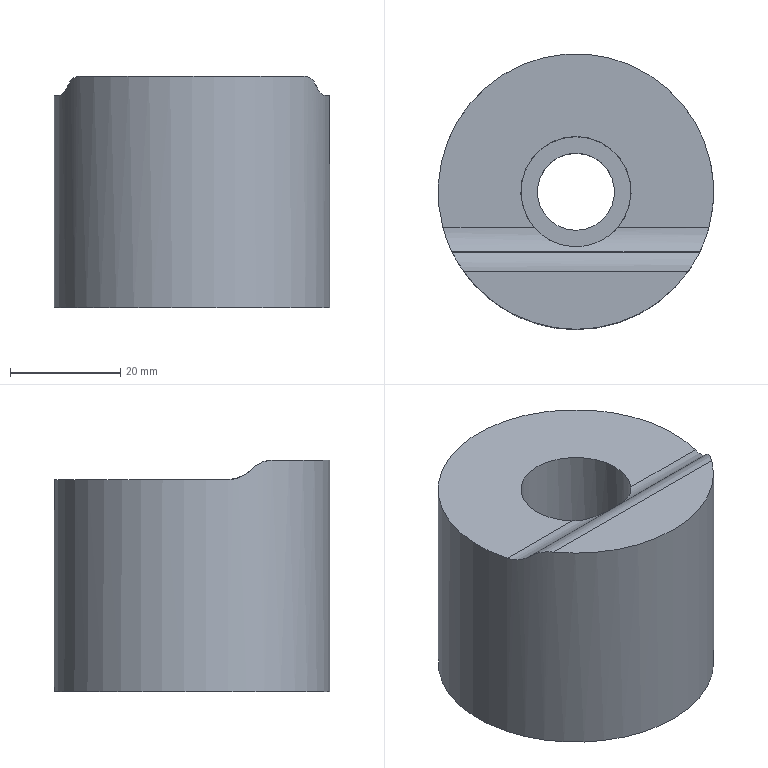Part | NX | features solid 2 | 1 solid | 10 faces | box 50 x 50 x 42.008 mm | volume 68335 mm3 | cylinder 5 | plane 5 | commonest cylinder face diameters 10 x1 12 x1 14 x1 20 x1 50 x1
STEP:
#1=CARTESIAN_POINT('',(-225.,485.,50.));
#2=VERTEX_POINT('',#1);
#3=CARTESIAN_POINT('',(-225.,510.,50.));
#4=DIRECTION('',(0.,0.,1.));
#5=DIRECTION('',(0.,-1.,0.));
#6=AXIS2_PLACEMENT_3D('',#3,#4,#5);
#7=CIRCLE('',#6,25.);
#8=EDGE_CURVE('',#2,#2,#7,.T.);
#9=ORIENTED_EDGE('',*,*,#8,.T.);
#10=EDGE_LOOP('',(#9));
#11=FACE_BOUND('',#10,.T.);
#12=CARTESIAN_POINT('',(-245.311,495.423,92.008));
#13=VERTEX_POINT('',#12);
#14=CARTESIAN_POINT('',(-204.689,495.423,92.008));
#15=VERTEX_POINT('',#14);
#16=CARTESIAN_POINT('',(-225.,510.,92.008));
#17=DIRECTION('',(0.,0.,1.));
#18=DIRECTION('',(0.,-1.,0.));
#19=AXIS2_PLACEMENT_3D('',#16,#17,#18);
#20=CIRCLE('',#19,25.);
#21=EDGE_CURVE('',#13,#15,#20,.T.);
#22=ORIENTED_EDGE('',*,*,#21,.F.);
#23=CARTESIAN_POINT('',(-247.454,499.009,90.492));
#24=VERTEX_POINT('',#23);
#25=CARTESIAN_POINT('',(-247.454,499.009,90.492));
#26=CARTESIAN_POINT('',(-246.96,497.999,91.532));
#27=CARTESIAN_POINT('',(-246.201,496.664,92.008));
#28=CARTESIAN_POINT('',(-245.311,495.423,92.008));
#29=B_SPLINE_CURVE_WITH_KNOTS('',3,(#25,#26,#27,#28),.UNSPECIFIED.,.F.,.F.,(4,4),(0.,0.004522),.UNSPECIFIED.);
#30=EDGE_CURVE('',#24,#13,#29,.T.);
#31=ORIENTED_EDGE('',*,*,#30,.F.);
#32=CARTESIAN_POINT('',(-247.533,499.171,90.326));
#33=VERTEX_POINT('',#32);
#34=CARTESIAN_POINT('',(-225.,510.,79.184));
#35=DIRECTION('',(0.,-0.7171,-0.697));
#36=DIRECTION('',(0.,0.697,-0.7171));
#37=AXIS2_PLACEMENT_3D('',#34,#35,#36);
#38=ELLIPSE('',#37,35.87,25.);
#39=EDGE_CURVE('',#24,#33,#38,.T.);
#40=ORIENTED_EDGE('',*,*,#39,.T.);
#41=CARTESIAN_POINT('',(-249.133,503.474,88.508));
#42=VERTEX_POINT('',#41);
#43=CARTESIAN_POINT('',(-247.533,499.171,90.326));
#44=CARTESIAN_POINT('',(-248.073,500.295,89.169));
#45=CARTESIAN_POINT('',(-248.689,501.831,88.508));
#46=CARTESIAN_POINT('',(-249.133,503.474,88.508));
#47=B_SPLINE_CURVE_WITH_KNOTS('',3,(#43,#44,#45,#46),.UNSPECIFIED.,.F.,.F.,(4,4),(0.,0.005031),.UNSPECIFIED.);
#48=EDGE_CURVE('',#33,#42,#47,.T.);
#49=ORIENTED_EDGE('',*,*,#48,.T.);
#50=CARTESIAN_POINT('',(-200.867,503.474,88.508));
#51=VERTEX_POINT('',#50);
#52=CARTESIAN_POINT('',(-225.,510.,88.508));
#53=DIRECTION('',(0.,0.,1.));
#54=DIRECTION('',(0.,-1.,0.));
#55=AXIS2_PLACEMENT_3D('',#52,#53,#54);
#56=CIRCLE('',#55,25.);
#57=EDGE_CURVE('',#51,#42,#56,.T.);
#58=ORIENTED_EDGE('',*,*,#57,.F.);
#59=CARTESIAN_POINT('',(-202.467,499.171,90.326));
#60=VERTEX_POINT('',#59);
#61=CARTESIAN_POINT('',(-200.867,503.474,88.508));
#62=CARTESIAN_POINT('',(-201.311,501.831,88.508));
#63=CARTESIAN_POINT('',(-201.927,500.294,89.17));
#64=CARTESIAN_POINT('',(-202.467,499.171,90.326));
#65=B_SPLINE_CURVE_WITH_KNOTS('',3,(#61,#62,#63,#64),.UNSPECIFIED.,.F.,.F.,(4,4),(0.,0.005028),.UNSPECIFIED.);
#66=EDGE_CURVE('',#51,#60,#65,.T.);
#67=ORIENTED_EDGE('',*,*,#66,.T.);
#68=CARTESIAN_POINT('',(-202.546,499.009,90.492));
#69=VERTEX_POINT('',#68);
#70=CARTESIAN_POINT('',(-225.,510.,79.184));
#71=DIRECTION('',(0.,-0.7171,-0.697));
#72=DIRECTION('',(0.,0.697,-0.7171));
#73=AXIS2_PLACEMENT_3D('',#70,#71,#72);
#74=ELLIPSE('',#73,35.87,25.);
#75=EDGE_CURVE('',#60,#69,#74,.T.);
#76=ORIENTED_EDGE('',*,*,#75,.T.);
#77=CARTESIAN_POINT('',(-204.689,495.423,92.008));
#78=CARTESIAN_POINT('',(-203.796,496.669,92.008));
#79=CARTESIAN_POINT('',(-203.043,497.993,91.538));
#80=CARTESIAN_POINT('',(-202.546,499.009,90.492));
#81=B_SPLINE_CURVE_WITH_KNOTS('',3,(#77,#78,#79,#80),.UNSPECIFIED.,.F.,.F.,(4,4),(0.,0.004516),.UNSPECIFIED.);
#82=EDGE_CURVE('',#15,#69,#81,.T.);
#83=ORIENTED_EDGE('',*,*,#82,.F.);
#84=EDGE_LOOP('',(#22,#31,#40,#49,#58,#67,#76,#83));
#85=FACE_BOUND('',#84,.T.);
#86=CARTESIAN_POINT('',(-225.,510.,100.));
#87=DIRECTION('',(0.,0.,-1.));
#88=DIRECTION('',(0.,1.,0.));
#89=AXIS2_PLACEMENT_3D('',#86,#87,#88);
#90=CYLINDRICAL_SURFACE('',#89,25.);
#91=ADVANCED_FACE('',(#11,#85),#90,.T.);
#92=CARTESIAN_POINT('',(-225.,503.,50.));
#93=VERTEX_POINT('',#92);
#94=CARTESIAN_POINT('',(-225.,510.,50.));
#95=DIRECTION('',(0.,0.,1.));
#96=DIRECTION('',(0.,-1.,0.));
#97=AXIS2_PLACEMENT_3D('',#94,#95,#96);
#98=CIRCLE('',#97,7.);
#99=EDGE_CURVE('',#93,#93,#98,.T.);
#100=ORIENTED_EDGE('',*,*,#99,.T.);
#101=EDGE_LOOP('',(#100));
#102=FACE_BOUND('',#101,.T.);
#103=ORIENTED_EDGE('',*,*,#8,.F.);
#104=EDGE_LOOP('',(#103));
#105=FACE_BOUND('',#104,.T.);
#106=CARTESIAN_POINT('',(-225.,510.,50.));
#107=DIRECTION('',(0.,0.,1.));
#108=DIRECTION('',(0.,-1.,0.));
#109=AXIS2_PLACEMENT_3D('',#106,#107,#108);
#110=PLANE('',#109);
#111=ADVANCED_FACE('',(#102,#105),#110,.F.);
#112=CARTESIAN_POINT('',(-204.689,495.423,92.008));
#113=CARTESIAN_POINT('',(-218.23,495.423,92.008));
#114=CARTESIAN_POINT('',(-231.77,495.423,92.008));
#115=CARTESIAN_POINT('',(-245.311,495.423,92.008));
#116=B_SPLINE_CURVE_WITH_KNOTS('',3,(#112,#113,#114,#115),.UNSPECIFIED.,.F.,.F.,(4,4),(0.7307,0.8175),.UNSPECIFIED.);
#117=EDGE_CURVE('',#15,#13,#116,.T.);
#118=ORIENTED_EDGE('',*,*,#117,.T.);
#119=ORIENTED_EDGE('',*,*,#21,.T.);
#120=EDGE_LOOP('',(#118,#119));
#121=FACE_BOUND('',#120,.T.);
#122=CARTESIAN_POINT('',(575.068,183.357,92.008));
#123=DIRECTION('',(0.,0.,1.));
#124=DIRECTION('',(0.,-1.,0.));
#125=AXIS2_PLACEMENT_3D('',#122,#123,#124);
#126=PLANE('',#125);
#127=ADVANCED_FACE('',(#121),#126,.T.);
#128=ORIENTED_EDGE('',*,*,#75,.F.);
#129=CARTESIAN_POINT('',(-247.533,499.171,90.326));
#130=CARTESIAN_POINT('',(-232.511,499.171,90.326));
#131=CARTESIAN_POINT('',(-217.489,499.171,90.326));
#132=CARTESIAN_POINT('',(-202.467,499.171,90.326));
#133=B_SPLINE_CURVE_WITH_KNOTS('',3,(#129,#130,#131,#132),.UNSPECIFIED.,.F.,.F.,(4,4),(0.1782,0.2748),.UNSPECIFIED.);
#134=EDGE_CURVE('',#33,#60,#133,.T.);
#135=ORIENTED_EDGE('',*,*,#134,.F.);
#136=ORIENTED_EDGE('',*,*,#39,.F.);
#137=CARTESIAN_POINT('',(-202.546,499.009,90.492));
#138=CARTESIAN_POINT('',(-217.515,499.009,90.492));
#139=CARTESIAN_POINT('',(-232.485,499.009,90.492));
#140=CARTESIAN_POINT('',(-247.454,499.009,90.492));
#141=B_SPLINE_CURVE_WITH_KNOTS('',3,(#137,#138,#139,#140),.UNSPECIFIED.,.F.,.F.,(4,4),(0.7254,0.8216),.UNSPECIFIED.);
#142=EDGE_CURVE('',#69,#24,#141,.T.);
#143=ORIENTED_EDGE('',*,*,#142,.F.);
#144=EDGE_LOOP('',(#128,#135,#136,#143));
#145=FACE_BOUND('',#144,.T.);
#146=CARTESIAN_POINT('',(-141.622,759.809,-177.845));
#147=DIRECTION('',(0.,-0.7171,-0.697));
#148=DIRECTION('',(0.,0.697,-0.7171));
#149=AXIS2_PLACEMENT_3D('',#146,#147,#148);
#150=PLANE('',#149);
#151=ADVANCED_FACE('',(#145),#150,.F.);
#152=ORIENTED_EDGE('',*,*,#117,.F.);
#153=ORIENTED_EDGE('',*,*,#82,.T.);
#154=ORIENTED_EDGE('',*,*,#142,.T.);
#155=ORIENTED_EDGE('',*,*,#30,.T.);
#156=EDGE_LOOP('',(#152,#153,#154,#155));
#157=FACE_BOUND('',#156,.T.);
#158=CARTESIAN_POINT('',(-6000330.729,495.423,87.008));
#159=DIRECTION('',(1.,0.,0.));
#160=DIRECTION('',(0.,0.,1.));
#161=AXIS2_PLACEMENT_3D('',#158,#159,#160);
#162=CYLINDRICAL_SURFACE('',#161,5.);
#163=ADVANCED_FACE('',(#157),#162,.T.);
#164=ORIENTED_EDGE('',*,*,#48,.F.);
#165=ORIENTED_EDGE('',*,*,#134,.T.);
#166=ORIENTED_EDGE('',*,*,#66,.F.);
#167=CARTESIAN_POINT('',(-217.423,503.474,88.508));
#168=VERTEX_POINT('',#167);
#169=CARTESIAN_POINT('',(-217.423,503.474,88.508));
#170=CARTESIAN_POINT('',(-211.905,503.474,88.508));
#171=CARTESIAN_POINT('',(-206.386,503.474,88.508));
#172=CARTESIAN_POINT('',(-200.867,503.474,88.508));
#173=B_SPLINE_CURVE_WITH_KNOTS('',3,(#169,#170,#171,#172),.UNSPECIFIED.,.F.,.F.,(4,4),(0.2427,0.2782),.UNSPECIFIED.);
#174=EDGE_CURVE('',#51,#168,#173,.F.);
#175=ORIENTED_EDGE('',*,*,#174,.T.);
#176=CARTESIAN_POINT('',(-232.577,503.474,88.508));
#177=VERTEX_POINT('',#176);
#178=CARTESIAN_POINT('',(-232.577,503.474,88.508));
#179=CARTESIAN_POINT('',(-231.621,502.365,88.508));
#180=CARTESIAN_POINT('',(-229.312,500.641,89.103));
#181=CARTESIAN_POINT('',(-225.005,499.681,89.871));
#182=CARTESIAN_POINT('',(-220.692,500.637,89.104));
#183=CARTESIAN_POINT('',(-218.378,502.366,88.508));
#184=CARTESIAN_POINT('',(-217.423,503.474,88.508));
#185=B_SPLINE_CURVE_WITH_KNOTS('',3,(#178,#179,#180,#181,#182,#183,#184),.UNSPECIFIED.,.F.,.F.,(4,1,1,1,4),(0.,0.004314,0.008627,0.01294,0.01725),.UNSPECIFIED.);
#186=EDGE_CURVE('',#177,#168,#185,.T.);
#187=ORIENTED_EDGE('',*,*,#186,.F.);
#188=CARTESIAN_POINT('',(-249.133,503.474,88.508));
#189=CARTESIAN_POINT('',(-243.614,503.474,88.508));
#190=CARTESIAN_POINT('',(-238.095,503.474,88.508));
#191=CARTESIAN_POINT('',(-232.577,503.474,88.508));
#192=B_SPLINE_CURVE_WITH_KNOTS('',3,(#188,#189,#190,#191),.UNSPECIFIED.,.F.,.F.,(4,4),(0.1747,0.2102),.UNSPECIFIED.);
#193=EDGE_CURVE('',#177,#42,#192,.F.);
#194=ORIENTED_EDGE('',*,*,#193,.T.);
#195=EDGE_LOOP('',(#164,#165,#166,#175,#187,#194));
#196=FACE_BOUND('',#195,.T.);
#197=CARTESIAN_POINT('',(6000135.646,503.474,94.508));
#198=DIRECTION('',(-1.,0.,0.));
#199=DIRECTION('',(0.,0.,-1.));
#200=AXIS2_PLACEMENT_3D('',#197,#198,#199);
#201=CYLINDRICAL_SURFACE('',#200,6.);
#202=ADVANCED_FACE('',(#196),#201,.F.);
#203=ORIENTED_EDGE('',*,*,#174,.F.);
#204=ORIENTED_EDGE('',*,*,#57,.T.);
#205=ORIENTED_EDGE('',*,*,#193,.F.);
#206=CARTESIAN_POINT('',(-225.,510.,88.508));
#207=DIRECTION('',(0.,0.,1.));
#208=DIRECTION('',(0.,-1.,0.));
#209=AXIS2_PLACEMENT_3D('',#206,#207,#208);
#210=CIRCLE('',#209,10.);
#211=EDGE_CURVE('',#177,#168,#210,.F.);
#212=ORIENTED_EDGE('',*,*,#211,.T.);
#213=EDGE_LOOP('',(#203,#204,#205,#212));
#214=FACE_BOUND('',#213,.T.);
#215=CARTESIAN_POINT('',(-123.101,672.26,88.508));
#216=DIRECTION('',(0.,0.,1.));
#217=DIRECTION('',(0.,-1.,0.));
#218=AXIS2_PLACEMENT_3D('',#215,#216,#217);
#219=PLANE('',#218);
#220=ADVANCED_FACE('',(#214),#219,.T.);
#221=CARTESIAN_POINT('',(-225.,517.,70.));
#222=VERTEX_POINT('',#221);
#223=CARTESIAN_POINT('',(-225.,510.,70.));
#224=DIRECTION('',(0.,0.,-1.));
#225=DIRECTION('',(0.,1.,0.));
#226=AXIS2_PLACEMENT_3D('',#223,#224,#225);
#227=CIRCLE('',#226,7.);
#228=EDGE_CURVE('',#222,#222,#227,.T.);
#229=ORIENTED_EDGE('',*,*,#228,.T.);
#230=EDGE_LOOP('',(#229));
#231=FACE_BOUND('',#230,.T.);
#232=CARTESIAN_POINT('',(-225.,520.,70.));
#233=VERTEX_POINT('',#232);
#234=CARTESIAN_POINT('',(-225.,510.,70.));
#235=DIRECTION('',(0.,0.,-1.));
#236=DIRECTION('',(0.,1.,0.));
#237=AXIS2_PLACEMENT_3D('',#234,#235,#236);
#238=CIRCLE('',#237,10.);
#239=EDGE_CURVE('',#233,#233,#238,.T.);
#240=ORIENTED_EDGE('',*,*,#239,.F.);
#241=EDGE_LOOP('',(#240));
#242=FACE_BOUND('',#241,.T.);
#243=CARTESIAN_POINT('',(-225.,510.,70.));
#244=DIRECTION('',(0.,0.,-1.));
#245=DIRECTION('',(0.,1.,0.));
#246=AXIS2_PLACEMENT_3D('',#243,#244,#245);
#247=PLANE('',#246);
#248=ADVANCED_FACE('',(#231,#242),#247,.F.);
#249=ORIENTED_EDGE('',*,*,#211,.F.);
#250=ORIENTED_EDGE('',*,*,#186,.T.);
#251=EDGE_LOOP('',(#249,#250));
#252=FACE_BOUND('',#251,.T.);
#253=ORIENTED_EDGE('',*,*,#239,.T.);
#254=EDGE_LOOP('',(#253));
#255=FACE_BOUND('',#254,.T.);
#256=CARTESIAN_POINT('',(-225.,510.,130.));
#257=DIRECTION('',(0.,0.,-1.));
#258=DIRECTION('',(0.,1.,0.));
#259=AXIS2_PLACEMENT_3D('',#256,#257,#258);
#260=CYLINDRICAL_SURFACE('',#259,10.);
#261=ADVANCED_FACE('',(#252,#255),#260,.F.);
#262=ORIENTED_EDGE('',*,*,#228,.F.);
#263=EDGE_LOOP('',(#262));
#264=FACE_BOUND('',#263,.T.);
#265=ORIENTED_EDGE('',*,*,#99,.F.);
#266=EDGE_LOOP('',(#265));
#267=FACE_BOUND('',#266,.T.);
#268=CARTESIAN_POINT('',(-225.,510.,70.));
#269=DIRECTION('',(0.,0.,-1.));
#270=DIRECTION('',(0.,1.,0.));
#271=AXIS2_PLACEMENT_3D('',#268,#269,#270);
#272=CYLINDRICAL_SURFACE('',#271,7.);
#273=ADVANCED_FACE('',(#264,#267),#272,.F.);
#274=CLOSED_SHELL('',(#91,#111,#127,#151,#163,#202,#220,#248,#261,#273));
#275=MANIFOLD_SOLID_BREP('',#274);
#276=(LENGTH_UNIT()NAMED_UNIT(*)SI_UNIT(.MILLI.,.METRE.));
#277=UNCERTAINTY_MEASURE_WITH_UNIT(LENGTH_MEASURE(0.0508),#276,'','');
#278=(NAMED_UNIT(*)PLANE_ANGLE_UNIT()SI_UNIT($,.RADIAN.));
#279=(NAMED_UNIT(*)SI_UNIT($,.STERADIAN.)SOLID_ANGLE_UNIT());
#280=(GEOMETRIC_REPRESENTATION_CONTEXT(3)GLOBAL_UNCERTAINTY_ASSIGNED_CONTEXT((#277))GLOBAL_UNIT_ASSIGNED_CONTEXT((#276,#278,#279))REPRESENTATION_CONTEXT('',''));
#281=ADVANCED_BREP_SHAPE_REPRESENTATION('',(#275),#280);